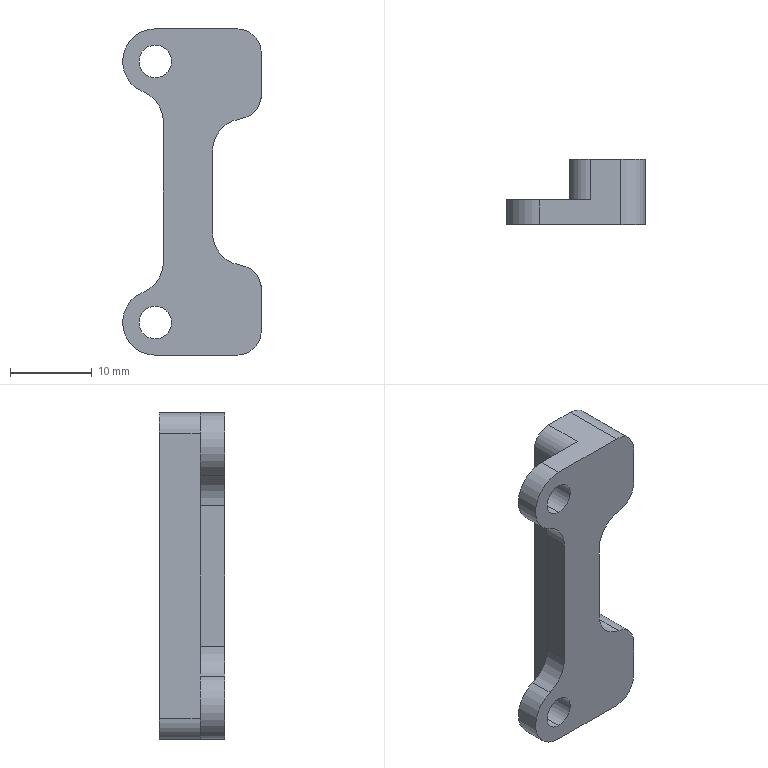NC program | Mastercam | posted with a generic post | part box 17 x 8 x 40 mm
Lines 7656 to 8055 of 8055:
(4 CHM |TOOL - 7|DIA. OFF. - 7|LEN. - 7|TOOL DIA. - 4.)
N5494 T7 M6
N5496 G0 G54 G90 X-16. Y4.5 C0. B0. S6000 M3
N5498 G43 H7 Z45.
N5500 G81 G98 Z-5.7 R-4. F200.
N5502 X16.
N5504 G80
N5506 Z50.
N5508 X-21.737 Y.944
N5510 Z15.154
N5512 Z5.154
N5514 G1 Z-4.846 F600.
N5516 X-21.728 Z-4.966 F1000.
N5518 X-21.7 Z-5.084
N5520 X-21.602 Z-5.311
N5522 X-21.46 Z-5.52
N5524 X-21.295 Z-5.705
N5526 X-21.232 Y.961 Z-5.768
N5528 X-21.175 Y1.007 Z-5.825
N5530 X-21.124 Y1.076 Z-5.876
N5532 X-21.082 Y1.163 Z-5.918
N5534 X-21.022 Y1.366 Z-5.978
N5536 X-21.001 Y1.569 Z-5.999
N5538 Y2.
N5540 X-20.994 Y3.25 Z-6.006
N5542 Y4.519
N5544 X-20.98 Y4.873
N5546 X-20.938 Y5.243
N5548 X-20.869 Y5.608
N5550 X-20.773 Y5.968
N5552 X-20.651 Y6.318
N5554 X-20.503 Y6.658
N5556 X-20.33 Y6.987
N5558 X-20.133 Y7.303
N5560 X-19.913 Y7.603
N5562 X-19.671 Y7.885
N5564 X-19.409 Y8.149
N5566 X-19.127 Y8.393
N5568 X-18.829 Y8.615
N5570 X-18.514 Y8.814
N5572 X-18.186 Y8.989
N5574 X-17.846 Y9.139
N5576 X-17.495 Y9.264
N5578 X-17.136 Y9.362
N5580 X-16.77 Y9.433
N5582 X-16.4 Y9.477
N5584 X-16.029 Y9.493
N5586 X-15.657 Y9.482
N5588 X-15.287 Y9.442
N5590 X-14.921 Y9.375
N5592 X-14.561 Y9.282
N5594 X-14.209 Y9.161
N5596 X-13.867 Y9.015
N5598 X-13.536 Y8.843
N5600 X-13.22 Y8.648
N5602 X-12.919 Y8.429
N5604 X-12.636 Y8.19
N5606 X-12.371 Y7.93
N5608 X-12.126 Y7.651
N5610 X-11.902 Y7.353
N5612 X-11.701 Y7.04
N5614 X-11.523 Y6.712
N5616 X-11.28 Y6.169
N5618 X-11.174 Y5.975
N5620 X-11.053 Y5.787
N5622 X-10.919 Y5.608
N5624 X-10.772 Y5.44
N5626 X-10.614 Y5.284
N5628 X-10.444 Y5.14
N5630 X-10.263 Y5.008
N5632 X-10.074 Y4.89
N5634 X-9.876 Y4.786
N5636 X-9.672 Y4.698
N5638 X-9.463 Y4.625
N5640 X-9.248 Y4.568
N5642 X-9.029 Y4.527
N5644 X-8.807 Y4.502
N5646 X-8.565 Y4.494
N5648 X-7.358
N5650 X-6.131
N5652 X-4.905
N5654 X-3.679
N5656 X-2.453
N5658 X-1.226
N5660 X0.
N5662 X1.226
N5664 X2.453
N5666 X3.679
N5668 X4.905
N5670 X6.131
N5672 X7.358
N5674 X8.565
N5676 X8.807 Y4.502
N5678 X9.029 Y4.527
N5680 X9.248 Y4.568
N5682 X9.463 Y4.625
N5684 X9.672 Y4.698
N5686 X9.876 Y4.786
N5688 X10.074 Y4.89
N5690 X10.263 Y5.008
N5692 X10.444 Y5.14
N5694 X10.614 Y5.284
N5696 X10.772 Y5.44
N5698 X10.919 Y5.608
N5700 X11.053 Y5.787
N5702 X11.174 Y5.975
N5704 X11.28 Y6.169
N5706 X11.523 Y6.712
N5708 X11.701 Y7.04
N5710 X11.902 Y7.353
N5712 X12.126 Y7.651
N5714 X12.371 Y7.93
N5716 X12.636 Y8.19
N5718 X12.919 Y8.429
N5720 X13.22 Y8.648
N5722 X13.536 Y8.843
N5724 X13.867 Y9.015
N5726 X14.209 Y9.161
N5728 X14.561 Y9.282
N5730 X14.921 Y9.375
N5732 X15.287 Y9.442
N5734 X15.657 Y9.482
N5736 X16.029 Y9.493
N5738 X16.4 Y9.477
N5740 X16.77 Y9.433
N5742 X17.136 Y9.362
N5744 X17.495 Y9.264
N5746 X17.846 Y9.139
N5748 X18.186 Y8.989
N5750 X18.514 Y8.814
N5752 X18.829 Y8.615
N5754 X19.127 Y8.393
N5756 X19.409 Y8.149
N5758 X19.671 Y7.885
N5760 X19.913 Y7.603
N5762 X20.133 Y7.303
N5764 X20.33 Y6.987
N5766 X20.503 Y6.658
N5768 X20.651 Y6.318
N5770 X20.773 Y5.968
N5772 X20.869 Y5.608
N5774 X20.938 Y5.243
N5776 X20.98 Y4.873
N5778 X20.994 Y4.519
N5780 Y3.25
N5782 X21.001 Y2. Z-5.999
N5784 Y1.569
N5786 X21.022 Y1.366 Z-5.978
N5788 X21.082 Y1.163 Z-5.918
N5790 X21.124 Y1.076 Z-5.876
N5792 X21.175 Y1.007 Z-5.825
N5794 X21.232 Y.961 Z-5.768
N5796 X21.295 Y.944 Z-5.705
N5798 X21.46 Z-5.52
N5800 X21.602 Z-5.311
N5802 X21.7 Z-5.084
N5804 X21.728 Z-4.966
N5806 X21.737 Z-4.846
N5808 G0 Z5.154
N5810 Z15.154
N5812 Z50.
N5814 X-.75 Y2.628
N5816 Z20.378
N5818 Z10.378
N5820 G1 Z.378 F600.
N5822 Y2.616 Z.234 F1000.
N5824 Y2.583 Z.092
N5826 Y2.532 Z-.046
N5828 Y2.465 Z-.18
N5830 Y2.295 Z-.431
N5832 Y2.097 Z-.653
N5834 X-.73 Y2.021 Z-.729
N5836 X-.675 Y1.952 Z-.798
N5838 X-.592 Y1.892 Z-.858
N5840 X-.488 Y1.841 Z-.909
N5842 X-.369 Y1.8 Z-.95
N5844 X-.244 Y1.769 Z-.981
N5846 X-.118 Y1.75 Z-1.
N5848 X0. Y1.744 Z-1.006
N5850 X1.25
N5852 X2.5
N5854 X3.75
N5856 X5.
N5858 X6.25
N5860 X7.5
N5862 X8.75
N5864 X10.
N5866 X11.25
N5868 X12.5
N5870 X13.75
N5872 X15.
N5874 X16.25
N5876 X17.524 Y1.743
N5878 X17.825 Y1.728
N5880 X18.145 Y1.684
N5882 X18.459 Y1.609
N5884 X18.764 Y1.507
N5886 X19.058 Y1.377
N5888 X19.338 Y1.22
N5890 X19.604 Y1.038
N5892 X19.853 Y.831
N5894 X20.081 Y.603
N5896 X20.288 Y.354
N5898 X20.47 Y.088
N5900 X20.627 Y-.192
N5902 X20.757 Y-.486
N5904 X20.859 Y-.791
N5906 X20.934 Y-1.105
N5908 X20.978 Y-1.425
N5910 X20.993 Y-1.726
N5912 X20.994 Y-3.
N5914 Y-4.25
N5916 X20.993 Y-5.521
N5918 X20.979 Y-5.833
N5920 X20.939 Y-6.16
N5922 X20.871 Y-6.483
N5924 X20.776 Y-6.799
N5926 X20.656 Y-7.105
N5928 X20.512 Y-7.4
N5930 X20.343 Y-7.683
N5932 X20.151 Y-7.952
N5934 X19.938 Y-8.204
N5936 X19.704 Y-8.438
N5938 X19.452 Y-8.651
N5940 X19.183 Y-8.843
N5942 X18.9 Y-9.012
N5944 X18.605 Y-9.156
N5946 X18.299 Y-9.276
N5948 X17.983 Y-9.371
N5950 X17.66 Y-9.439
N5952 X17.333 Y-9.479
N5954 X17.021 Y-9.493
N5956 X15.979 Y-9.494
N5958 X14.958
N5960 X13.937
N5962 X12.915
N5964 X11.867 Y-9.493
N5966 X11.551 Y-9.476
N5968 X11.224 Y-9.431
N5970 X10.902 Y-9.359
N5972 X10.587 Y-9.262
N5974 X10.283 Y-9.139
N5976 X9.989 Y-8.991
N5978 X9.708 Y-8.819
N5980 X9.442 Y-8.624
N5982 X9.192 Y-8.407
N5984 X8.961 Y-8.171
N5986 X8.75 Y-7.916
N5988 X8.562 Y-7.646
N5990 X8.397 Y-7.363
N5992 X8.257 Y-7.068
N5994 X8.14 Y-6.763
N5996 X8.047 Y-6.446
N5998 X7.985 Y-6.145
N6000 X7.936 Y-5.856
N6002 X7.883 Y-5.651
N6004 X7.815 Y-5.447
N6006 X7.733 Y-5.249
N6008 X7.637 Y-5.057
N6010 X7.528 Y-4.874
N6012 X7.406 Y-4.699
N6014 X7.272 Y-4.532
N6016 X7.125 Y-4.375
N6018 X6.968 Y-4.229
N6020 X6.8 Y-4.093
N6022 X6.623 Y-3.971
N6024 X6.438 Y-3.861
N6026 X6.247 Y-3.765
N6028 X6.05 Y-3.683
N6030 X5.848 Y-3.616
N6032 X5.64 Y-3.563
N6034 X5.429 Y-3.525
N6036 X5.216 Y-3.502
N6038 X4.982 Y-3.494
N6040 X3.75
N6042 X2.5
N6044 X1.25
N6046 X0.
N6048 X-1.25
N6050 X-2.5
N6052 X-3.75
N6054 X-4.982
N6056 X-5.216 Y-3.502
N6058 X-5.429 Y-3.525
N6060 X-5.64 Y-3.563
N6062 X-5.848 Y-3.616
N6064 X-6.05 Y-3.683
N6066 X-6.247 Y-3.765
N6068 X-6.438 Y-3.861
N6070 X-6.623 Y-3.971
N6072 X-6.8 Y-4.093
N6074 X-6.968 Y-4.229
N6076 X-7.125 Y-4.375
N6078 X-7.272 Y-4.532
N6080 X-7.406 Y-4.699
N6082 X-7.528 Y-4.874
N6084 X-7.637 Y-5.057
N6086 X-7.733 Y-5.249
N6088 X-7.815 Y-5.447
N6090 X-7.883 Y-5.651
N6092 X-7.936 Y-5.856
N6094 X-7.985 Y-6.145
N6096 X-8.047 Y-6.446
N6098 X-8.14 Y-6.763
N6100 X-8.257 Y-7.068
N6102 X-8.397 Y-7.363
N6104 X-8.562 Y-7.646
N6106 X-8.75 Y-7.916
N6108 X-8.961 Y-8.171
N6110 X-9.192 Y-8.407
N6112 X-9.442 Y-8.624
N6114 X-9.708 Y-8.819
N6116 X-9.989 Y-8.991
N6118 X-10.283 Y-9.139
N6120 X-10.587 Y-9.262
N6122 X-10.902 Y-9.359
N6124 X-11.224 Y-9.431
N6126 X-11.554 Y-9.476
N6128 X-11.904 Y-9.493
N6130 X-12.943 Y-9.494
N6132 X-13.957
N6134 X-14.971
N6136 X-15.986
N6138 X-17.021 Y-9.493
N6140 X-17.333 Y-9.479
N6142 X-17.66 Y-9.439
N6144 X-17.983 Y-9.371
N6146 X-18.299 Y-9.276
N6148 X-18.605 Y-9.156
N6150 X-18.9 Y-9.012
N6152 X-19.183 Y-8.843
N6154 X-19.452 Y-8.651
N6156 X-19.704 Y-8.438
N6158 X-19.938 Y-8.204
N6160 X-20.151 Y-7.952
N6162 X-20.343 Y-7.683
N6164 X-20.512 Y-7.4
N6166 X-20.656 Y-7.105
N6168 X-20.776 Y-6.799
N6170 X-20.871 Y-6.483
N6172 X-20.939 Y-6.16
N6174 X-20.979 Y-5.833
N6176 X-20.993 Y-5.521
N6178 X-20.994 Y-4.25
N6180 Y-3.
N6182 X-20.993 Y-1.726
N6184 X-20.978 Y-1.425
N6186 X-20.934 Y-1.105
N6188 X-20.859 Y-.791
N6190 X-20.757 Y-.486
N6192 X-20.627 Y-.192
N6194 X-20.47 Y.088
N6196 X-20.288 Y.354
N6198 X-20.081 Y.603
N6200 X-19.853 Y.831
N6202 X-19.604 Y1.038
N6204 X-19.338 Y1.22
N6206 X-19.058 Y1.377
N6208 X-18.764 Y1.507
N6210 X-18.459 Y1.609
N6212 X-18.145 Y1.684
N6214 X-17.825 Y1.728
N6216 X-17.524 Y1.743
N6218 X-16.25 Y1.744
N6220 X-15.
N6222 X-13.75
N6224 X-12.5
N6226 X-11.25
N6228 X-10.
N6230 X-8.75
N6232 X-7.5
N6234 X-6.25
N6236 X-5.
N6238 X-3.75
N6240 X-2.5
N6242 X-1.25
N6244 X0.
N6246 X.118 Y1.75 Z-1.
N6248 X.244 Y1.769 Z-.981
N6250 X.369 Y1.8 Z-.95
N6252 X.488 Y1.841 Z-.909
N6254 X.592 Y1.892 Z-.858
N6256 X.675 Y1.952 Z-.798
N6258 X.73 Y2.021 Z-.729
N6260 X.75 Y2.097 Z-.653
N6262 Y2.295 Z-.431
N6264 Y2.465 Z-.18
N6266 Y2.532 Z-.046
N6268 Y2.583 Z.092
N6270 Y2.616 Z.234
N6272 Y2.628 Z.378
N6274 G0 Z10.378
N6276 Z20.378
N6278 Z50.
N6280 M5
N6282 G0 G28 G91 Z0.
N6284 G0 G28 X0. Y0.
N6286 G28
N6288 M30
%